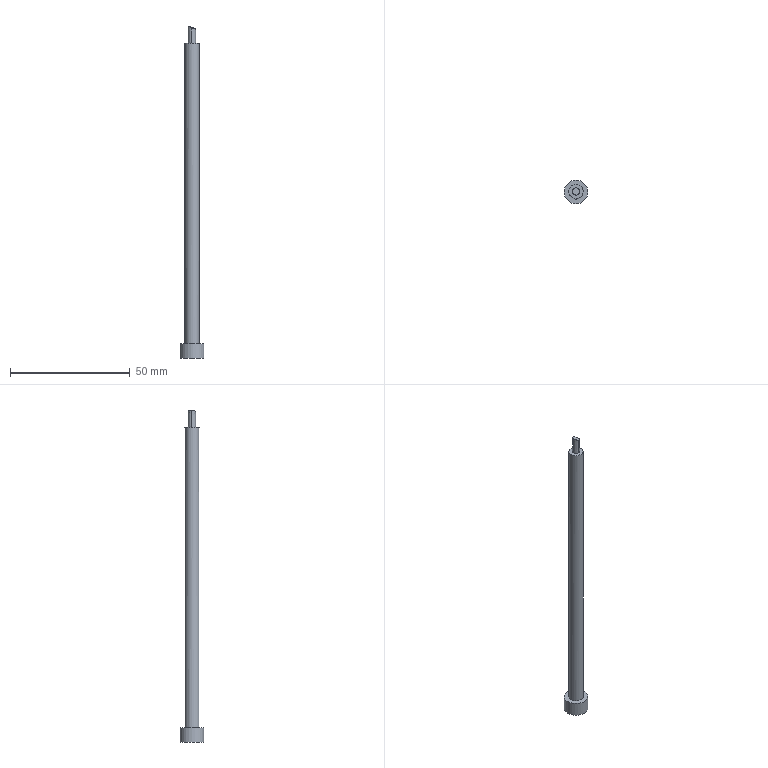Part | STEP file | 车灯-后视镜_id662_x_t | 1 solid | 10 faces | box 10 x 10 x 138.616 mm | volume 4062 mm3 | spline 5 | plane 3 | cylinder 2 | commonest cylinder face diameters 6 x1 10 x1
STEP:
#1=CARTESIAN_POINT('',(53.384,22.013,-68.));
#2=VERTEX_POINT('',#1);
#3=CARTESIAN_POINT('',(50.384,22.013,-68.));
#4=DIRECTION('',(0.,0.,-1.));
#5=DIRECTION('',(1.,0.,0.));
#6=AXIS2_PLACEMENT_3D('',#3,#4,#5);
#7=CIRCLE('',#6,3.);
#8=EDGE_CURVE('',#2,#2,#7,.T.);
#9=ORIENTED_EDGE('',*,*,#8,.F.);
#10=EDGE_LOOP('',(#9));
#11=FACE_BOUND('',#10,.T.);
#12=CARTESIAN_POINT('',(53.379,21.851,57.333));
#13=VERTEX_POINT('',#12);
#14=CARTESIAN_POINT('',(50.384,22.013,57.333));
#15=DIRECTION('',(0.0001201,-0.000006508,-1.));
#16=DIRECTION('',(0.9985,-0.05413,0.0001202));
#17=AXIS2_PLACEMENT_3D('',#14,#15,#16);
#18=ELLIPSE('',#17,3.,3.);
#19=EDGE_CURVE('',#13,#13,#18,.T.);
#20=ORIENTED_EDGE('',*,*,#19,.T.);
#21=EDGE_LOOP('',(#20));
#22=FACE_BOUND('',#21,.T.);
#23=CARTESIAN_POINT('',(50.384,22.013,57.333));
#24=DIRECTION('',(0.,0.,1.));
#25=DIRECTION('',(1.,0.,0.));
#26=AXIS2_PLACEMENT_3D('',#23,#24,#25);
#27=CYLINDRICAL_SURFACE('',#26,3.);
#28=ADVANCED_FACE('',(#11,#22),#27,.T.);
#29=CARTESIAN_POINT('',(49.364,20.914,64.294));
#30=VERTEX_POINT('',#29);
#31=CARTESIAN_POINT('',(49.837,20.611,64.064));
#32=VERTEX_POINT('',#31);
#33=CARTESIAN_POINT('',(49.384,20.895,64.285));
#34=CARTESIAN_POINT('',(49.52,20.772,64.217));
#35=CARTESIAN_POINT('',(49.671,20.678,64.144));
#36=CARTESIAN_POINT('',(49.838,20.611,64.066));
#37=B_SPLINE_CURVE_WITH_KNOTS('',3,(#33,#34,#35,#36),.UNSPECIFIED.,.F.,.F.,(4,4),(0.,1.),.UNSPECIFIED.);
#38=EDGE_CURVE('',#30,#32,#37,.T.);
#39=ORIENTED_EDGE('',*,*,#38,.T.);
#40=CARTESIAN_POINT('',(50.383,20.506,63.821));
#41=VERTEX_POINT('',#40);
#42=CARTESIAN_POINT('',(49.838,20.611,64.066));
#43=CARTESIAN_POINT('',(50.014,20.54,63.984));
#44=CARTESIAN_POINT('',(50.196,20.505,63.903));
#45=CARTESIAN_POINT('',(50.383,20.506,63.821));
#46=B_SPLINE_CURVE_WITH_KNOTS('',3,(#42,#43,#44,#45),.UNSPECIFIED.,.F.,.F.,(4,4),(0.,1.),.UNSPECIFIED.);
#47=EDGE_CURVE('',#32,#41,#46,.T.);
#48=ORIENTED_EDGE('',*,*,#47,.T.);
#49=CARTESIAN_POINT('',(50.518,20.512,63.763));
#50=VERTEX_POINT('',#49);
#51=CARTESIAN_POINT('',(50.383,20.506,63.821));
#52=CARTESIAN_POINT('',(50.428,20.508,63.802));
#53=CARTESIAN_POINT('',(50.473,20.51,63.782));
#54=CARTESIAN_POINT('',(50.518,20.512,63.763));
#55=B_SPLINE_CURVE_WITH_KNOTS('',3,(#51,#52,#53,#54),.UNSPECIFIED.,.F.,.F.,(4,4),(0.,1.),.UNSPECIFIED.);
#56=EDGE_CURVE('',#41,#50,#55,.T.);
#57=ORIENTED_EDGE('',*,*,#56,.T.);
#58=CARTESIAN_POINT('',(51.013,20.648,63.557));
#59=VERTEX_POINT('',#58);
#60=CARTESIAN_POINT('',(50.518,20.512,63.763));
#61=CARTESIAN_POINT('',(50.683,20.557,63.694));
#62=CARTESIAN_POINT('',(50.848,20.603,63.625));
#63=CARTESIAN_POINT('',(51.013,20.648,63.556));
#64=B_SPLINE_CURVE_WITH_KNOTS('',3,(#60,#61,#62,#63),.UNSPECIFIED.,.F.,.F.,(4,4),(0.,1.),.UNSPECIFIED.);
#65=EDGE_CURVE('',#50,#59,#64,.T.);
#66=ORIENTED_EDGE('',*,*,#65,.T.);
#67=CARTESIAN_POINT('',(51.89,22.013,63.277));
#68=VERTEX_POINT('',#67);
#69=CARTESIAN_POINT('',(51.013,20.648,63.556));
#70=CARTESIAN_POINT('',(51.535,20.896,63.345));
#71=CARTESIAN_POINT('',(51.879,21.412,63.23));
#72=CARTESIAN_POINT('',(51.89,22.013,63.277));
#73=B_SPLINE_CURVE_WITH_KNOTS('',3,(#69,#70,#71,#72),.UNSPECIFIED.,.F.,.F.,(4,4),(0.,1.),.UNSPECIFIED.);
#74=EDGE_CURVE('',#59,#68,#73,.T.);
#75=ORIENTED_EDGE('',*,*,#74,.T.);
#76=CARTESIAN_POINT('',(51.423,23.093,63.592));
#77=VERTEX_POINT('',#76);
#78=CARTESIAN_POINT('',(51.89,22.013,63.277));
#79=CARTESIAN_POINT('',(51.887,22.43,63.314));
#80=CARTESIAN_POINT('',(51.731,22.79,63.418));
#81=CARTESIAN_POINT('',(51.42,23.093,63.585));
#82=B_SPLINE_CURVE_WITH_KNOTS('',3,(#78,#79,#80,#81),.UNSPECIFIED.,.F.,.F.,(4,4),(0.,1.),.UNSPECIFIED.);
#83=EDGE_CURVE('',#68,#77,#82,.T.);
#84=ORIENTED_EDGE('',*,*,#83,.T.);
#85=CARTESIAN_POINT('',(51.035,23.367,63.788));
#86=VERTEX_POINT('',#85);
#87=CARTESIAN_POINT('',(51.42,23.093,63.585));
#88=CARTESIAN_POINT('',(51.305,23.205,63.647));
#89=CARTESIAN_POINT('',(51.176,23.297,63.713));
#90=CARTESIAN_POINT('',(51.033,23.368,63.783));
#91=B_SPLINE_CURVE_WITH_KNOTS('',3,(#87,#88,#89,#90),.UNSPECIFIED.,.F.,.F.,(4,4),(0.,1.),.UNSPECIFIED.);
#92=EDGE_CURVE('',#77,#86,#91,.T.);
#93=ORIENTED_EDGE('',*,*,#92,.T.);
#94=CARTESIAN_POINT('',(50.383,23.521,64.086));
#95=VERTEX_POINT('',#94);
#96=CARTESIAN_POINT('',(51.033,23.368,63.783));
#97=CARTESIAN_POINT('',(50.826,23.47,63.885));
#98=CARTESIAN_POINT('',(50.609,23.521,63.986));
#99=CARTESIAN_POINT('',(50.383,23.521,64.086));
#100=B_SPLINE_CURVE_WITH_KNOTS('',3,(#96,#97,#98,#99),.UNSPECIFIED.,.F.,.F.,(4,4),(0.,1.),.UNSPECIFIED.);
#101=EDGE_CURVE('',#86,#95,#100,.T.);
#102=ORIENTED_EDGE('',*,*,#101,.T.);
#103=CARTESIAN_POINT('',(50.241,23.514,64.147));
#104=VERTEX_POINT('',#103);
#105=CARTESIAN_POINT('',(50.383,23.521,64.086));
#106=CARTESIAN_POINT('',(50.336,23.518,64.106));
#107=CARTESIAN_POINT('',(50.289,23.516,64.127));
#108=CARTESIAN_POINT('',(50.241,23.514,64.147));
#109=B_SPLINE_CURVE_WITH_KNOTS('',3,(#105,#106,#107,#108),.UNSPECIFIED.,.F.,.F.,(4,4),(0.,1.),.UNSPECIFIED.);
#110=EDGE_CURVE('',#95,#104,#109,.T.);
#111=ORIENTED_EDGE('',*,*,#110,.T.);
#112=CARTESIAN_POINT('',(49.749,23.376,64.348));
#113=VERTEX_POINT('',#112);
#114=CARTESIAN_POINT('',(50.241,23.514,64.147));
#115=CARTESIAN_POINT('',(50.078,23.468,64.215));
#116=CARTESIAN_POINT('',(49.914,23.422,64.282));
#117=CARTESIAN_POINT('',(49.749,23.376,64.349));
#118=B_SPLINE_CURVE_WITH_KNOTS('',3,(#114,#115,#116,#117),.UNSPECIFIED.,.F.,.F.,(4,4),(0.,1.),.UNSPECIFIED.);
#119=EDGE_CURVE('',#104,#113,#118,.T.);
#120=ORIENTED_EDGE('',*,*,#119,.T.);
#121=CARTESIAN_POINT('',(48.875,22.013,64.6));
#122=VERTEX_POINT('',#121);
#123=CARTESIAN_POINT('',(49.749,23.376,64.349));
#124=CARTESIAN_POINT('',(49.177,23.103,64.572));
#125=CARTESIAN_POINT('',(48.883,22.648,64.653));
#126=CARTESIAN_POINT('',(48.875,22.013,64.6));
#127=B_SPLINE_CURVE_WITH_KNOTS('',3,(#123,#124,#125,#126),.UNSPECIFIED.,.F.,.F.,(4,4),(0.,1.),.UNSPECIFIED.);
#128=EDGE_CURVE('',#113,#122,#127,.T.);
#129=ORIENTED_EDGE('',*,*,#128,.T.);
#130=CARTESIAN_POINT('',(48.875,22.013,64.6));
#131=CARTESIAN_POINT('',(48.878,21.592,64.561));
#132=CARTESIAN_POINT('',(49.036,21.232,64.463));
#133=CARTESIAN_POINT('',(49.344,20.932,64.306));
#134=B_SPLINE_CURVE_WITH_KNOTS('',3,(#130,#131,#132,#133),.UNSPECIFIED.,.F.,.F.,(4,4),(0.,1.),.UNSPECIFIED.);
#135=EDGE_CURVE('',#122,#30,#134,.T.);
#136=ORIENTED_EDGE('',*,*,#135,.T.);
#137=EDGE_LOOP('',(#39,#48,#57,#66,#75,#84,#93,#102,#111,#120,#129,#136));
#138=FACE_OUTER_BOUND('',#137,.T.);
#139=CARTESIAN_POINT('',(48.83,20.498,64.482));
#140=CARTESIAN_POINT('',(49.869,20.49,64.05));
#141=CARTESIAN_POINT('',(50.886,20.482,63.605));
#142=CARTESIAN_POINT('',(51.881,20.475,63.147));
#143=CARTESIAN_POINT('',(48.847,21.513,64.568));
#144=CARTESIAN_POINT('',(49.887,21.505,64.134));
#145=CARTESIAN_POINT('',(50.905,21.498,63.688));
#146=CARTESIAN_POINT('',(51.901,21.49,63.227));
#147=CARTESIAN_POINT('',(48.863,22.531,64.652));
#148=CARTESIAN_POINT('',(49.904,22.523,64.217));
#149=CARTESIAN_POINT('',(50.924,22.515,63.769));
#150=CARTESIAN_POINT('',(51.921,22.508,63.306));
#151=CARTESIAN_POINT('',(48.878,23.552,64.734));
#152=CARTESIAN_POINT('',(49.92,23.544,64.297));
#153=CARTESIAN_POINT('',(50.941,23.536,63.847));
#154=CARTESIAN_POINT('',(51.939,23.528,63.383));
#155=B_SPLINE_SURFACE_WITH_KNOTS('',3,3,((#139,#140,#141,#142),(#143,#144,#145,#146),(#147,#148,#149,#150),(#151,#152,#153,#154)),.UNSPECIFIED.,.F.,.F.,.F.,(4,4),(4,4),(0.,1.),(0.,1.),.UNSPECIFIED.);
#156=ADVANCED_FACE('',(#138),#155,.F.);
#157=CARTESIAN_POINT('',(50.384,23.521,57.333));
#158=VERTEX_POINT('',#157);
#159=CARTESIAN_POINT('',(50.383,23.521,60.73));
#160=DIRECTION('',(0.0001192,-0.00000676,-1.));
#161=VECTOR('',#160,1.);
#162=LINE('',#159,#161);
#163=EDGE_CURVE('',#95,#158,#162,.T.);
#164=ORIENTED_EDGE('',*,*,#163,.T.);
#165=CARTESIAN_POINT('',(48.876,22.013,57.333));
#166=VERTEX_POINT('',#165);
#167=CARTESIAN_POINT('',(50.384,23.521,57.333));
#168=CARTESIAN_POINT('',(49.563,23.521,57.333));
#169=CARTESIAN_POINT('',(48.876,22.834,57.333));
#170=CARTESIAN_POINT('',(48.876,22.013,57.333));
#171=B_SPLINE_CURVE_WITH_KNOTS('',3,(#167,#168,#169,#170),.UNSPECIFIED.,.F.,.F.,(4,4),(0.,1.),.UNSPECIFIED.);
#172=EDGE_CURVE('',#158,#166,#171,.T.);
#173=ORIENTED_EDGE('',*,*,#172,.T.);
#174=CARTESIAN_POINT('',(48.876,22.013,60.988));
#175=DIRECTION('',(-0.0001192,0.00000676,1.));
#176=VECTOR('',#175,1.);
#177=LINE('',#174,#176);
#178=EDGE_CURVE('',#166,#122,#177,.T.);
#179=ORIENTED_EDGE('',*,*,#178,.T.);
#180=ORIENTED_EDGE('',*,*,#128,.F.);
#181=ORIENTED_EDGE('',*,*,#119,.F.);
#182=ORIENTED_EDGE('',*,*,#110,.F.);
#183=EDGE_LOOP('',(#164,#173,#179,#180,#181,#182));
#184=FACE_OUTER_BOUND('',#183,.T.);
#185=CARTESIAN_POINT('',(48.876,22.013,57.333));
#186=CARTESIAN_POINT('',(48.876,22.013,59.775));
#187=CARTESIAN_POINT('',(48.876,22.013,62.218));
#188=CARTESIAN_POINT('',(48.875,22.013,64.661));
#189=CARTESIAN_POINT('',(48.876,22.834,57.333));
#190=CARTESIAN_POINT('',(48.876,22.834,59.775));
#191=CARTESIAN_POINT('',(48.876,22.834,62.218));
#192=CARTESIAN_POINT('',(48.875,22.834,64.661));
#193=CARTESIAN_POINT('',(49.563,23.521,57.333));
#194=CARTESIAN_POINT('',(49.563,23.521,59.775));
#195=CARTESIAN_POINT('',(49.562,23.521,62.218));
#196=CARTESIAN_POINT('',(49.562,23.521,64.661));
#197=CARTESIAN_POINT('',(50.384,23.521,57.333));
#198=CARTESIAN_POINT('',(50.383,23.521,59.776));
#199=CARTESIAN_POINT('',(50.383,23.521,62.218));
#200=CARTESIAN_POINT('',(50.383,23.521,64.661));
#201=B_SPLINE_SURFACE_WITH_KNOTS('',3,3,((#185,#186,#187,#188),(#189,#190,#191,#192),(#193,#194,#195,#196),(#197,#198,#199,#200)),.UNSPECIFIED.,.F.,.F.,.F.,(4,4),(4,4),(0.,1.),(0.,1.),.UNSPECIFIED.);
#202=ADVANCED_FACE('',(#184),#201,.F.);
#203=ORIENTED_EDGE('',*,*,#38,.F.);
#204=ORIENTED_EDGE('',*,*,#135,.F.);
#205=ORIENTED_EDGE('',*,*,#178,.F.);
#206=CARTESIAN_POINT('',(50.384,20.506,57.333));
#207=VERTEX_POINT('',#206);
#208=CARTESIAN_POINT('',(48.876,22.013,57.333));
#209=CARTESIAN_POINT('',(48.876,21.192,57.333));
#210=CARTESIAN_POINT('',(49.563,20.506,57.333));
#211=CARTESIAN_POINT('',(50.384,20.506,57.333));
#212=B_SPLINE_CURVE_WITH_KNOTS('',3,(#208,#209,#210,#211),.UNSPECIFIED.,.F.,.F.,(4,4),(0.,1.),.UNSPECIFIED.);
#213=EDGE_CURVE('',#166,#207,#212,.T.);
#214=ORIENTED_EDGE('',*,*,#213,.T.);
#215=CARTESIAN_POINT('',(50.383,20.506,60.988));
#216=DIRECTION('',(0.0001192,-0.00000676,-1.));
#217=VECTOR('',#216,1.);
#218=LINE('',#215,#217);
#219=EDGE_CURVE('',#41,#207,#218,.T.);
#220=ORIENTED_EDGE('',*,*,#219,.F.);
#221=ORIENTED_EDGE('',*,*,#47,.F.);
#222=EDGE_LOOP('',(#203,#204,#205,#214,#220,#221));
#223=FACE_OUTER_BOUND('',#222,.T.);
#224=CARTESIAN_POINT('',(50.384,20.506,57.333));
#225=CARTESIAN_POINT('',(50.383,20.506,59.77));
#226=CARTESIAN_POINT('',(50.383,20.506,62.207));
#227=CARTESIAN_POINT('',(50.383,20.506,64.644));
#228=CARTESIAN_POINT('',(49.563,20.506,57.333));
#229=CARTESIAN_POINT('',(49.563,20.506,59.77));
#230=CARTESIAN_POINT('',(49.562,20.506,62.207));
#231=CARTESIAN_POINT('',(49.562,20.506,64.644));
#232=CARTESIAN_POINT('',(48.876,21.192,57.333));
#233=CARTESIAN_POINT('',(48.876,21.192,59.77));
#234=CARTESIAN_POINT('',(48.876,21.192,62.207));
#235=CARTESIAN_POINT('',(48.875,21.192,64.643));
#236=CARTESIAN_POINT('',(48.876,22.013,57.333));
#237=CARTESIAN_POINT('',(48.876,22.013,59.77));
#238=CARTESIAN_POINT('',(48.876,22.013,62.207));
#239=CARTESIAN_POINT('',(48.875,22.013,64.643));
#240=B_SPLINE_SURFACE_WITH_KNOTS('',3,3,((#224,#225,#226,#227),(#228,#229,#230,#231),(#232,#233,#234,#235),(#236,#237,#238,#239)),.UNSPECIFIED.,.F.,.F.,.F.,(4,4),(4,4),(0.,1.),(0.,1.),.UNSPECIFIED.);
#241=ADVANCED_FACE('',(#223),#240,.F.);
#242=ORIENTED_EDGE('',*,*,#219,.T.);
#243=CARTESIAN_POINT('',(51.891,22.013,57.333));
#244=VERTEX_POINT('',#243);
#245=CARTESIAN_POINT('',(51.891,22.013,57.333));
#246=CARTESIAN_POINT('',(51.891,21.205,57.333));
#247=CARTESIAN_POINT('',(51.189,20.506,57.333));
#248=CARTESIAN_POINT('',(50.384,20.506,57.333));
#249=B_SPLINE_CURVE_WITH_KNOTS('',3,(#245,#246,#247,#248),.UNSPECIFIED.,.F.,.F.,(4,4),(0.,1.),.UNSPECIFIED.);
#250=EDGE_CURVE('',#244,#207,#249,.T.);
#251=ORIENTED_EDGE('',*,*,#250,.F.);
#252=CARTESIAN_POINT('',(51.891,22.013,60.73));
#253=DIRECTION('',(-0.0001192,0.00000676,1.));
#254=VECTOR('',#253,1.);
#255=LINE('',#252,#254);
#256=EDGE_CURVE('',#244,#68,#255,.T.);
#257=ORIENTED_EDGE('',*,*,#256,.T.);
#258=ORIENTED_EDGE('',*,*,#74,.F.);
#259=ORIENTED_EDGE('',*,*,#65,.F.);
#260=ORIENTED_EDGE('',*,*,#56,.F.);
#261=EDGE_LOOP('',(#242,#251,#257,#258,#259,#260));
#262=FACE_OUTER_BOUND('',#261,.T.);
#263=CARTESIAN_POINT('',(51.891,22.013,57.333));
#264=CARTESIAN_POINT('',(51.891,22.013,59.509));
#265=CARTESIAN_POINT('',(51.891,22.013,61.684));
#266=CARTESIAN_POINT('',(51.89,22.013,63.86));
#267=CARTESIAN_POINT('',(51.891,21.192,57.333));
#268=CARTESIAN_POINT('',(51.891,21.192,59.509));
#269=CARTESIAN_POINT('',(51.891,21.192,61.684));
#270=CARTESIAN_POINT('',(51.89,21.192,63.86));
#271=CARTESIAN_POINT('',(51.204,20.506,57.333));
#272=CARTESIAN_POINT('',(51.204,20.506,59.509));
#273=CARTESIAN_POINT('',(51.204,20.506,61.684));
#274=CARTESIAN_POINT('',(51.204,20.506,63.86));
#275=CARTESIAN_POINT('',(50.384,20.506,57.333));
#276=CARTESIAN_POINT('',(50.383,20.506,59.509));
#277=CARTESIAN_POINT('',(50.383,20.506,61.684));
#278=CARTESIAN_POINT('',(50.383,20.506,63.86));
#279=B_SPLINE_SURFACE_WITH_KNOTS('',3,3,((#263,#264,#265,#266),(#267,#268,#269,#270),(#271,#272,#273,#274),(#275,#276,#277,#278)),.UNSPECIFIED.,.F.,.F.,.F.,(4,4),(4,4),(0.,1.),(0.,1.),.UNSPECIFIED.);
#280=ADVANCED_FACE('',(#262),#279,.F.);
#281=ORIENTED_EDGE('',*,*,#92,.F.);
#282=ORIENTED_EDGE('',*,*,#83,.F.);
#283=ORIENTED_EDGE('',*,*,#256,.F.);
#284=CARTESIAN_POINT('',(51.891,22.013,57.333));
#285=CARTESIAN_POINT('',(51.891,22.834,57.333));
#286=CARTESIAN_POINT('',(51.204,23.521,57.333));
#287=CARTESIAN_POINT('',(50.384,23.521,57.333));
#288=B_SPLINE_CURVE_WITH_KNOTS('',3,(#284,#285,#286,#287),.UNSPECIFIED.,.F.,.F.,(4,4),(0.,1.),.UNSPECIFIED.);
#289=EDGE_CURVE('',#244,#158,#288,.T.);
#290=ORIENTED_EDGE('',*,*,#289,.T.);
#291=ORIENTED_EDGE('',*,*,#163,.F.);
#292=ORIENTED_EDGE('',*,*,#101,.F.);
#293=EDGE_LOOP('',(#281,#282,#283,#290,#291,#292));
#294=FACE_OUTER_BOUND('',#293,.T.);
#295=CARTESIAN_POINT('',(50.384,23.521,57.333));
#296=CARTESIAN_POINT('',(50.383,23.521,59.597));
#297=CARTESIAN_POINT('',(50.383,23.521,61.862));
#298=CARTESIAN_POINT('',(50.383,23.521,64.126));
#299=CARTESIAN_POINT('',(51.204,23.521,57.333));
#300=CARTESIAN_POINT('',(51.204,23.521,59.597));
#301=CARTESIAN_POINT('',(51.204,23.521,61.862));
#302=CARTESIAN_POINT('',(51.204,23.521,64.126));
#303=CARTESIAN_POINT('',(51.891,22.834,57.333));
#304=CARTESIAN_POINT('',(51.891,22.834,59.598));
#305=CARTESIAN_POINT('',(51.891,22.834,61.862));
#306=CARTESIAN_POINT('',(51.89,22.834,64.126));
#307=CARTESIAN_POINT('',(51.891,22.013,57.333));
#308=CARTESIAN_POINT('',(51.891,22.013,59.598));
#309=CARTESIAN_POINT('',(51.891,22.013,61.862));
#310=CARTESIAN_POINT('',(51.89,22.013,64.126));
#311=B_SPLINE_SURFACE_WITH_KNOTS('',3,3,((#295,#296,#297,#298),(#299,#300,#301,#302),(#303,#304,#305,#306),(#307,#308,#309,#310)),.UNSPECIFIED.,.F.,.F.,.F.,(4,4),(4,4),(0.,1.),(0.,1.),.UNSPECIFIED.);
#312=ADVANCED_FACE('',(#294),#311,.F.);
#313=ORIENTED_EDGE('',*,*,#289,.F.);
#314=ORIENTED_EDGE('',*,*,#250,.T.);
#315=ORIENTED_EDGE('',*,*,#213,.F.);
#316=ORIENTED_EDGE('',*,*,#172,.F.);
#317=EDGE_LOOP('',(#313,#314,#315,#316));
#318=FACE_BOUND('',#317,.T.);
#319=ORIENTED_EDGE('',*,*,#19,.F.);
#320=EDGE_LOOP('',(#319));
#321=FACE_BOUND('',#320,.T.);
#322=CARTESIAN_POINT('',(51.891,22.013,57.333));
#323=DIRECTION('',(0.0001201,-0.000006508,-1.));
#324=DIRECTION('',(-0.7071,0.7071,-0.00008949));
#325=AXIS2_PLACEMENT_3D('',#322,#323,#324);
#326=PLANE('',#325);
#327=ADVANCED_FACE('',(#318,#321),#326,.F.);
#328=ORIENTED_EDGE('',*,*,#8,.T.);
#329=EDGE_LOOP('',(#328));
#330=FACE_BOUND('',#329,.T.);
#331=CARTESIAN_POINT('',(45.384,22.013,-68.));
#332=VERTEX_POINT('',#331);
#333=CARTESIAN_POINT('',(50.384,22.013,-68.));
#334=DIRECTION('',(0.,0.,-1.));
#335=DIRECTION('',(-1.,0.,0.));
#336=AXIS2_PLACEMENT_3D('',#333,#334,#335);
#337=CIRCLE('',#336,5.);
#338=EDGE_CURVE('',#332,#332,#337,.T.);
#339=ORIENTED_EDGE('',*,*,#338,.F.);
#340=EDGE_LOOP('',(#339));
#341=FACE_BOUND('',#340,.T.);
#342=CARTESIAN_POINT('',(50.384,22.013,-68.));
#343=DIRECTION('',(0.,0.,1.));
#344=DIRECTION('',(1.,0.,0.));
#345=AXIS2_PLACEMENT_3D('',#342,#343,#344);
#346=PLANE('',#345);
#347=ADVANCED_FACE('',(#330,#341),#346,.T.);
#348=ORIENTED_EDGE('',*,*,#338,.T.);
#349=EDGE_LOOP('',(#348));
#350=FACE_BOUND('',#349,.T.);
#351=CARTESIAN_POINT('',(55.384,22.013,-74.));
#352=VERTEX_POINT('',#351);
#353=CARTESIAN_POINT('',(50.384,22.013,-74.));
#354=DIRECTION('',(0.,0.,1.));
#355=DIRECTION('',(1.,0.,0.));
#356=AXIS2_PLACEMENT_3D('',#353,#354,#355);
#357=CIRCLE('',#356,5.);
#358=EDGE_CURVE('',#352,#352,#357,.T.);
#359=ORIENTED_EDGE('',*,*,#358,.T.);
#360=EDGE_LOOP('',(#359));
#361=FACE_BOUND('',#360,.T.);
#362=CARTESIAN_POINT('',(50.384,22.013,-74.));
#363=DIRECTION('',(0.,0.,1.));
#364=DIRECTION('',(1.,0.,0.));
#365=AXIS2_PLACEMENT_3D('',#362,#363,#364);
#366=CYLINDRICAL_SURFACE('',#365,5.);
#367=ADVANCED_FACE('',(#350,#361),#366,.T.);
#368=ORIENTED_EDGE('',*,*,#358,.F.);
#369=EDGE_LOOP('',(#368));
#370=FACE_OUTER_BOUND('',#369,.T.);
#371=CARTESIAN_POINT('',(15.,0.,-74.));
#372=DIRECTION('',(0.,0.,-1.));
#373=DIRECTION('',(-1.,0.,0.));
#374=AXIS2_PLACEMENT_3D('',#371,#372,#373);
#375=PLANE('',#374);
#376=ADVANCED_FACE('',(#370),#375,.T.);
#377=CLOSED_SHELL('',(#28,#156,#202,#241,#280,#312,#327,#347,#367,#376));
#378=MANIFOLD_SOLID_BREP('',#377);
#379=(LENGTH_UNIT()NAMED_UNIT(*)SI_UNIT(.MILLI.,.METRE.));
#380=UNCERTAINTY_MEASURE_WITH_UNIT(LENGTH_MEASURE(0.08898),#379,'','');
#381=(NAMED_UNIT(*)PLANE_ANGLE_UNIT()SI_UNIT($,.RADIAN.));
#382=PLANE_ANGLE_MEASURE_WITH_UNIT(PLANE_ANGLE_MEASURE(0.01745),#381);
#383=DIMENSIONAL_EXPONENTS(0.,0.,0.,0.,0.,0.,0.);
#384=(CONVERSION_BASED_UNIT('DEGREE',#382)NAMED_UNIT(#383)PLANE_ANGLE_UNIT());
#385=(NAMED_UNIT(*)SI_UNIT($,.STERADIAN.)SOLID_ANGLE_UNIT());
#386=(GEOMETRIC_REPRESENTATION_CONTEXT(3)GLOBAL_UNCERTAINTY_ASSIGNED_CONTEXT((#380))GLOBAL_UNIT_ASSIGNED_CONTEXT((#379,#384,#385))REPRESENTATION_CONTEXT('',''));
#387=ADVANCED_BREP_SHAPE_REPRESENTATION('',(#378),#386);